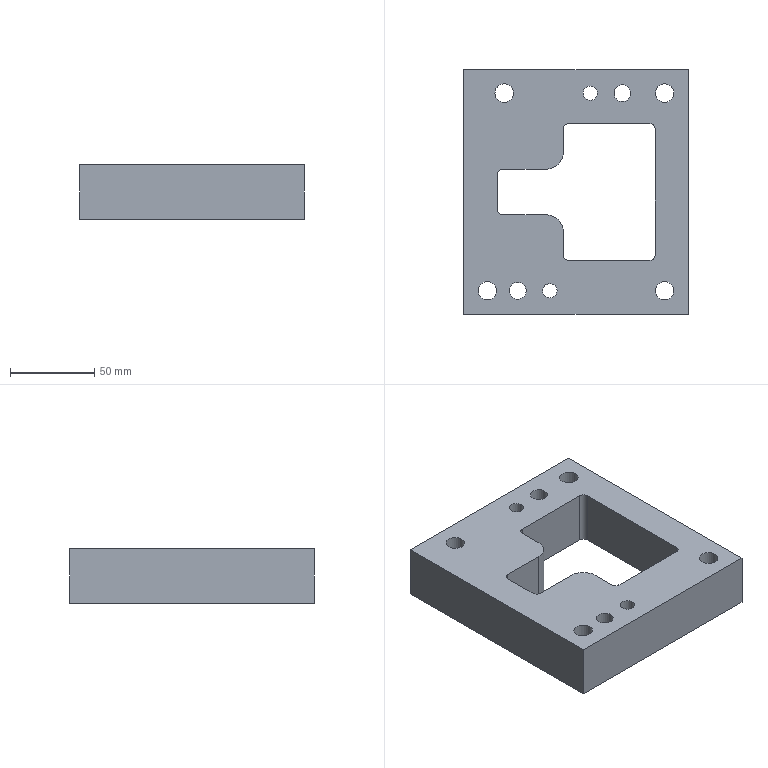Part | STEP file | lll_id3514_x_t | 1 solid | 38 faces | box 133 x 145 x 32 mm | volume 413987 mm3 | cylinder 20 | plane 18 | commonest cylinder face diameters 6 x6 11 x4 17 x4 8.506 x2 10 x2 20 x2
STEP:
#1=CARTESIAN_POINT('',(3776.,72.5,92.5));
#2=VERTEX_POINT('',#1);
#3=CARTESIAN_POINT('',(3909.,72.5,92.5));
#4=VERTEX_POINT('',#3);
#5=CARTESIAN_POINT('',(3841.5,72.5,92.5));
#6=DIRECTION('',(1.,0.,0.));
#7=VECTOR('',#6,1.);
#8=LINE('',#5,#7);
#9=EDGE_CURVE('',#2,#4,#8,.T.);
#10=ORIENTED_EDGE('',*,*,#9,.F.);
#11=CARTESIAN_POINT('',(3776.,-72.5,92.5));
#12=VERTEX_POINT('',#11);
#13=CARTESIAN_POINT('',(3776.,0.00007613,92.5));
#14=DIRECTION('',(0.,1.,0.));
#15=VECTOR('',#14,1.);
#16=LINE('',#13,#15);
#17=EDGE_CURVE('',#12,#2,#16,.T.);
#18=ORIENTED_EDGE('',*,*,#17,.F.);
#19=CARTESIAN_POINT('',(3909.,-72.5,92.5));
#20=VERTEX_POINT('',#19);
#21=CARTESIAN_POINT('',(3841.5,-72.5,92.5));
#22=DIRECTION('',(-1.,0.,0.));
#23=VECTOR('',#22,1.);
#24=LINE('',#21,#23);
#25=EDGE_CURVE('',#20,#12,#24,.T.);
#26=ORIENTED_EDGE('',*,*,#25,.F.);
#27=CARTESIAN_POINT('',(3909.,0.00007613,92.5));
#28=DIRECTION('',(0.,-1.,0.));
#29=VECTOR('',#28,1.);
#30=LINE('',#27,#29);
#31=EDGE_CURVE('',#4,#20,#30,.T.);
#32=ORIENTED_EDGE('',*,*,#31,.F.);
#33=EDGE_LOOP('',(#10,#18,#26,#32));
#34=FACE_BOUND('',#33,.T.);
#35=CARTESIAN_POINT('',(3889.5,58.5,92.5));
#36=VERTEX_POINT('',#35);
#37=CARTESIAN_POINT('',(3895.,58.5,92.5));
#38=DIRECTION('',(0.,0.,1.));
#39=DIRECTION('',(-1.,0.,0.));
#40=AXIS2_PLACEMENT_3D('',#37,#38,#39);
#41=CIRCLE('',#40,5.5);
#42=EDGE_CURVE('',#36,#36,#41,.T.);
#43=ORIENTED_EDGE('',*,*,#42,.F.);
#44=EDGE_LOOP('',(#43));
#45=FACE_BOUND('',#44,.T.);
#46=CARTESIAN_POINT('',(3784.5,-58.5,92.5));
#47=VERTEX_POINT('',#46);
#48=CARTESIAN_POINT('',(3790.,-58.5,92.5));
#49=DIRECTION('',(0.,0.,1.));
#50=DIRECTION('',(-1.,0.,0.));
#51=AXIS2_PLACEMENT_3D('',#48,#49,#50);
#52=CIRCLE('',#51,5.5);
#53=EDGE_CURVE('',#47,#47,#52,.T.);
#54=ORIENTED_EDGE('',*,*,#53,.F.);
#55=EDGE_LOOP('',(#54));
#56=FACE_BOUND('',#55,.T.);
#57=CARTESIAN_POINT('',(3794.5,58.5,92.5));
#58=VERTEX_POINT('',#57);
#59=CARTESIAN_POINT('',(3800.,58.5,92.5));
#60=DIRECTION('',(0.,0.,1.));
#61=DIRECTION('',(-1.,0.,0.));
#62=AXIS2_PLACEMENT_3D('',#59,#60,#61);
#63=CIRCLE('',#62,5.5);
#64=EDGE_CURVE('',#58,#58,#63,.T.);
#65=ORIENTED_EDGE('',*,*,#64,.F.);
#66=EDGE_LOOP('',(#65));
#67=FACE_BOUND('',#66,.T.);
#68=CARTESIAN_POINT('',(3889.5,-58.5,92.5));
#69=VERTEX_POINT('',#68);
#70=CARTESIAN_POINT('',(3895.,-58.5,92.5));
#71=DIRECTION('',(0.,0.,1.));
#72=DIRECTION('',(-1.,0.,0.));
#73=AXIS2_PLACEMENT_3D('',#70,#71,#72);
#74=CIRCLE('',#73,5.5);
#75=EDGE_CURVE('',#69,#69,#74,.T.);
#76=ORIENTED_EDGE('',*,*,#75,.F.);
#77=EDGE_LOOP('',(#76));
#78=FACE_BOUND('',#77,.T.);
#79=CARTESIAN_POINT('',(3865.,58.5,92.5));
#80=VERTEX_POINT('',#79);
#81=CARTESIAN_POINT('',(3870.,58.5,92.5));
#82=DIRECTION('',(0.,0.,1.));
#83=DIRECTION('',(-1.,0.,0.));
#84=AXIS2_PLACEMENT_3D('',#81,#82,#83);
#85=CIRCLE('',#84,5.);
#86=EDGE_CURVE('',#80,#80,#85,.T.);
#87=ORIENTED_EDGE('',*,*,#86,.F.);
#88=EDGE_LOOP('',(#87));
#89=FACE_BOUND('',#88,.T.);
#90=CARTESIAN_POINT('',(3803.,-58.5,92.5));
#91=VERTEX_POINT('',#90);
#92=CARTESIAN_POINT('',(3808.,-58.5,92.5));
#93=DIRECTION('',(0.,0.,1.));
#94=DIRECTION('',(-1.,0.,0.));
#95=AXIS2_PLACEMENT_3D('',#92,#93,#94);
#96=CIRCLE('',#95,5.);
#97=EDGE_CURVE('',#91,#91,#96,.T.);
#98=ORIENTED_EDGE('',*,*,#97,.F.);
#99=EDGE_LOOP('',(#98));
#100=FACE_BOUND('',#99,.T.);
#101=CARTESIAN_POINT('',(3846.747,58.5,92.5));
#102=VERTEX_POINT('',#101);
#103=CARTESIAN_POINT('',(3851.,58.5,92.5));
#104=DIRECTION('',(0.,0.,1.));
#105=DIRECTION('',(-1.,0.,0.));
#106=AXIS2_PLACEMENT_3D('',#103,#104,#105);
#107=CIRCLE('',#106,4.253);
#108=EDGE_CURVE('',#102,#102,#107,.T.);
#109=ORIENTED_EDGE('',*,*,#108,.F.);
#110=EDGE_LOOP('',(#109));
#111=FACE_BOUND('',#110,.T.);
#112=CARTESIAN_POINT('',(3822.747,-58.5,92.5));
#113=VERTEX_POINT('',#112);
#114=CARTESIAN_POINT('',(3827.,-58.5,92.5));
#115=DIRECTION('',(0.,0.,1.));
#116=DIRECTION('',(-1.,0.,0.));
#117=AXIS2_PLACEMENT_3D('',#114,#115,#116);
#118=CIRCLE('',#117,4.253);
#119=EDGE_CURVE('',#113,#113,#118,.T.);
#120=ORIENTED_EDGE('',*,*,#119,.F.);
#121=EDGE_LOOP('',(#120));
#122=FACE_BOUND('',#121,.T.);
#123=CARTESIAN_POINT('',(3796.,-10.5,92.5));
#124=VERTEX_POINT('',#123);
#125=CARTESIAN_POINT('',(3799.,-13.5,92.5));
#126=VERTEX_POINT('',#125);
#127=CARTESIAN_POINT('',(3799.,-10.5,92.5));
#128=DIRECTION('',(0.,0.,1.));
#129=DIRECTION('',(-1.,0.,0.));
#130=AXIS2_PLACEMENT_3D('',#127,#128,#129);
#131=CIRCLE('',#130,3.);
#132=EDGE_CURVE('',#124,#126,#131,.T.);
#133=ORIENTED_EDGE('',*,*,#132,.F.);
#134=CARTESIAN_POINT('',(3796.,10.5,92.5));
#135=VERTEX_POINT('',#134);
#136=CARTESIAN_POINT('',(3796.,236.7,92.5));
#137=DIRECTION('',(0.,1.,0.));
#138=VECTOR('',#137,1.);
#139=LINE('',#136,#138);
#140=EDGE_CURVE('',#124,#135,#139,.T.);
#141=ORIENTED_EDGE('',*,*,#140,.T.);
#142=CARTESIAN_POINT('',(3799.,13.5,92.5));
#143=VERTEX_POINT('',#142);
#144=CARTESIAN_POINT('',(3799.,10.5,92.5));
#145=DIRECTION('',(0.,0.,1.));
#146=DIRECTION('',(-1.,0.,0.));
#147=AXIS2_PLACEMENT_3D('',#144,#145,#146);
#148=CIRCLE('',#147,3.);
#149=EDGE_CURVE('',#143,#135,#148,.T.);
#150=ORIENTED_EDGE('',*,*,#149,.F.);
#151=CARTESIAN_POINT('',(3825.,13.5,92.5));
#152=VERTEX_POINT('',#151);
#153=CARTESIAN_POINT('',(3831.,13.5,92.5));
#154=DIRECTION('',(-1.,0.,0.));
#155=VECTOR('',#154,1.);
#156=LINE('',#153,#155);
#157=EDGE_CURVE('',#152,#143,#156,.T.);
#158=ORIENTED_EDGE('',*,*,#157,.F.);
#159=CARTESIAN_POINT('',(3835.,23.5,92.5));
#160=VERTEX_POINT('',#159);
#161=CARTESIAN_POINT('',(3825.,23.5,92.5));
#162=DIRECTION('',(0.,0.,-1.));
#163=DIRECTION('',(-1.,0.,0.));
#164=AXIS2_PLACEMENT_3D('',#161,#162,#163);
#165=CIRCLE('',#164,10.);
#166=EDGE_CURVE('',#160,#152,#165,.T.);
#167=ORIENTED_EDGE('',*,*,#166,.F.);
#168=CARTESIAN_POINT('',(3835.,37.5,92.5));
#169=VERTEX_POINT('',#168);
#170=CARTESIAN_POINT('',(3835.,38.,92.5));
#171=DIRECTION('',(0.,-1.,0.));
#172=VECTOR('',#171,1.);
#173=LINE('',#170,#172);
#174=EDGE_CURVE('',#169,#160,#173,.T.);
#175=ORIENTED_EDGE('',*,*,#174,.F.);
#176=CARTESIAN_POINT('',(3838.,40.5,92.5));
#177=VERTEX_POINT('',#176);
#178=CARTESIAN_POINT('',(3838.,37.5,92.5));
#179=DIRECTION('',(0.,0.,1.));
#180=DIRECTION('',(-1.,0.,0.));
#181=AXIS2_PLACEMENT_3D('',#178,#179,#180);
#182=CIRCLE('',#181,3.);
#183=EDGE_CURVE('',#177,#169,#182,.T.);
#184=ORIENTED_EDGE('',*,*,#183,.F.);
#185=CARTESIAN_POINT('',(3886.3,40.5,92.5));
#186=VERTEX_POINT('',#185);
#187=CARTESIAN_POINT('',(3587.234,40.5,92.5));
#188=DIRECTION('',(1.,0.,0.));
#189=VECTOR('',#188,1.);
#190=LINE('',#187,#189);
#191=EDGE_CURVE('',#177,#186,#190,.T.);
#192=ORIENTED_EDGE('',*,*,#191,.T.);
#193=CARTESIAN_POINT('',(3889.3,37.5,92.5));
#194=VERTEX_POINT('',#193);
#195=CARTESIAN_POINT('',(3886.3,37.5,92.5));
#196=DIRECTION('',(0.,0.,1.));
#197=DIRECTION('',(-1.,0.,0.));
#198=AXIS2_PLACEMENT_3D('',#195,#196,#197);
#199=CIRCLE('',#198,3.);
#200=EDGE_CURVE('',#194,#186,#199,.T.);
#201=ORIENTED_EDGE('',*,*,#200,.F.);
#202=CARTESIAN_POINT('',(3889.3,-37.5,92.5));
#203=VERTEX_POINT('',#202);
#204=CARTESIAN_POINT('',(3889.3,236.7,92.5));
#205=DIRECTION('',(0.,-1.,0.));
#206=VECTOR('',#205,1.);
#207=LINE('',#204,#206);
#208=EDGE_CURVE('',#194,#203,#207,.T.);
#209=ORIENTED_EDGE('',*,*,#208,.T.);
#210=CARTESIAN_POINT('',(3886.3,-40.5,92.5));
#211=VERTEX_POINT('',#210);
#212=CARTESIAN_POINT('',(3886.3,-37.5,92.5));
#213=DIRECTION('',(0.,0.,1.));
#214=DIRECTION('',(-1.,0.,0.));
#215=AXIS2_PLACEMENT_3D('',#212,#213,#214);
#216=CIRCLE('',#215,3.);
#217=EDGE_CURVE('',#211,#203,#216,.T.);
#218=ORIENTED_EDGE('',*,*,#217,.F.);
#219=CARTESIAN_POINT('',(3838.,-40.5,92.5));
#220=VERTEX_POINT('',#219);
#221=CARTESIAN_POINT('',(14362.883,-40.5,92.5));
#222=DIRECTION('',(1.,0.,0.));
#223=VECTOR('',#222,1.);
#224=LINE('',#221,#223);
#225=EDGE_CURVE('',#220,#211,#224,.T.);
#226=ORIENTED_EDGE('',*,*,#225,.F.);
#227=CARTESIAN_POINT('',(3835.,-37.5,92.5));
#228=VERTEX_POINT('',#227);
#229=CARTESIAN_POINT('',(3838.,-37.5,92.5));
#230=DIRECTION('',(0.,0.,1.));
#231=DIRECTION('',(-1.,0.,0.));
#232=AXIS2_PLACEMENT_3D('',#229,#230,#231);
#233=CIRCLE('',#232,3.);
#234=EDGE_CURVE('',#228,#220,#233,.T.);
#235=ORIENTED_EDGE('',*,*,#234,.F.);
#236=CARTESIAN_POINT('',(3835.,-23.5,92.5));
#237=VERTEX_POINT('',#236);
#238=CARTESIAN_POINT('',(3835.,236.7,92.5));
#239=DIRECTION('',(0.,1.,0.));
#240=VECTOR('',#239,1.);
#241=LINE('',#238,#240);
#242=EDGE_CURVE('',#228,#237,#241,.T.);
#243=ORIENTED_EDGE('',*,*,#242,.T.);
#244=CARTESIAN_POINT('',(3825.,-13.5,92.5));
#245=VERTEX_POINT('',#244);
#246=CARTESIAN_POINT('',(3825.,-23.5,92.5));
#247=DIRECTION('',(0.,0.,-1.));
#248=DIRECTION('',(-1.,0.,0.));
#249=AXIS2_PLACEMENT_3D('',#246,#247,#248);
#250=CIRCLE('',#249,10.);
#251=EDGE_CURVE('',#245,#237,#250,.T.);
#252=ORIENTED_EDGE('',*,*,#251,.F.);
#253=CARTESIAN_POINT('',(3587.234,-13.5,92.5));
#254=DIRECTION('',(-1.,0.,0.));
#255=VECTOR('',#254,1.);
#256=LINE('',#253,#255);
#257=EDGE_CURVE('',#245,#126,#256,.T.);
#258=ORIENTED_EDGE('',*,*,#257,.T.);
#259=EDGE_LOOP('',(#133,#141,#150,#158,#167,#175,#184,#192,#201,#209,#218,#226,#235,#243,#252,#258));
#260=FACE_BOUND('',#259,.T.);
#261=CARTESIAN_POINT('',(3841.5,0.00007613,92.5));
#262=DIRECTION('',(0.,0.,1.));
#263=DIRECTION('',(-1.,0.,0.));
#264=AXIS2_PLACEMENT_3D('',#261,#262,#263);
#265=PLANE('',#264);
#266=ADVANCED_FACE('',(#34,#45,#56,#67,#78,#89,#100,#111,#122,#260),#265,.T.);
#267=CARTESIAN_POINT('',(3889.3,-37.5,60.5));
#268=VERTEX_POINT('',#267);
#269=CARTESIAN_POINT('',(3886.3,-40.5,60.5));
#270=VERTEX_POINT('',#269);
#271=CARTESIAN_POINT('',(3886.3,-37.5,60.5));
#272=DIRECTION('',(0.,0.,-1.));
#273=DIRECTION('',(1.,0.,0.));
#274=AXIS2_PLACEMENT_3D('',#271,#272,#273);
#275=CIRCLE('',#274,3.);
#276=EDGE_CURVE('',#268,#270,#275,.T.);
#277=ORIENTED_EDGE('',*,*,#276,.F.);
#278=CARTESIAN_POINT('',(3889.3,37.5,60.5));
#279=VERTEX_POINT('',#278);
#280=CARTESIAN_POINT('',(3889.3,0.00007613,60.5));
#281=DIRECTION('',(0.,-1.,0.));
#282=VECTOR('',#281,1.);
#283=LINE('',#280,#282);
#284=EDGE_CURVE('',#279,#268,#283,.T.);
#285=ORIENTED_EDGE('',*,*,#284,.F.);
#286=CARTESIAN_POINT('',(3886.3,40.5,60.5));
#287=VERTEX_POINT('',#286);
#288=CARTESIAN_POINT('',(3886.3,37.5,60.5));
#289=DIRECTION('',(0.,0.,-1.));
#290=DIRECTION('',(1.,0.,0.));
#291=AXIS2_PLACEMENT_3D('',#288,#289,#290);
#292=CIRCLE('',#291,3.);
#293=EDGE_CURVE('',#287,#279,#292,.T.);
#294=ORIENTED_EDGE('',*,*,#293,.F.);
#295=CARTESIAN_POINT('',(3838.,40.5,60.5));
#296=VERTEX_POINT('',#295);
#297=CARTESIAN_POINT('',(3841.5,40.5,60.5));
#298=DIRECTION('',(1.,0.,0.));
#299=VECTOR('',#298,1.);
#300=LINE('',#297,#299);
#301=EDGE_CURVE('',#296,#287,#300,.T.);
#302=ORIENTED_EDGE('',*,*,#301,.F.);
#303=CARTESIAN_POINT('',(3835.,37.5,60.5));
#304=VERTEX_POINT('',#303);
#305=CARTESIAN_POINT('',(3838.,37.5,60.5));
#306=DIRECTION('',(0.,0.,-1.));
#307=DIRECTION('',(1.,0.,0.));
#308=AXIS2_PLACEMENT_3D('',#305,#306,#307);
#309=CIRCLE('',#308,3.);
#310=EDGE_CURVE('',#304,#296,#309,.T.);
#311=ORIENTED_EDGE('',*,*,#310,.F.);
#312=CARTESIAN_POINT('',(3835.,23.5,60.5));
#313=VERTEX_POINT('',#312);
#314=CARTESIAN_POINT('',(3835.,0.00007613,60.5));
#315=DIRECTION('',(0.,1.,0.));
#316=VECTOR('',#315,1.);
#317=LINE('',#314,#316);
#318=EDGE_CURVE('',#313,#304,#317,.T.);
#319=ORIENTED_EDGE('',*,*,#318,.F.);
#320=CARTESIAN_POINT('',(3825.,13.5,60.5));
#321=VERTEX_POINT('',#320);
#322=CARTESIAN_POINT('',(3825.,23.5,60.5));
#323=DIRECTION('',(0.,0.,-1.));
#324=DIRECTION('',(1.,0.,0.));
#325=AXIS2_PLACEMENT_3D('',#322,#323,#324);
#326=CIRCLE('',#325,10.);
#327=EDGE_CURVE('',#313,#321,#326,.T.);
#328=ORIENTED_EDGE('',*,*,#327,.T.);
#329=CARTESIAN_POINT('',(3799.,13.5,60.5));
#330=VERTEX_POINT('',#329);
#331=CARTESIAN_POINT('',(3841.5,13.5,60.5));
#332=DIRECTION('',(1.,0.,0.));
#333=VECTOR('',#332,1.);
#334=LINE('',#331,#333);
#335=EDGE_CURVE('',#330,#321,#334,.T.);
#336=ORIENTED_EDGE('',*,*,#335,.F.);
#337=CARTESIAN_POINT('',(3796.,10.5,60.5));
#338=VERTEX_POINT('',#337);
#339=CARTESIAN_POINT('',(3799.,10.5,60.5));
#340=DIRECTION('',(0.,0.,-1.));
#341=DIRECTION('',(1.,0.,0.));
#342=AXIS2_PLACEMENT_3D('',#339,#340,#341);
#343=CIRCLE('',#342,3.);
#344=EDGE_CURVE('',#338,#330,#343,.T.);
#345=ORIENTED_EDGE('',*,*,#344,.F.);
#346=CARTESIAN_POINT('',(3796.,-10.5,60.5));
#347=VERTEX_POINT('',#346);
#348=CARTESIAN_POINT('',(3796.,0.00007613,60.5));
#349=DIRECTION('',(0.,1.,0.));
#350=VECTOR('',#349,1.);
#351=LINE('',#348,#350);
#352=EDGE_CURVE('',#347,#338,#351,.T.);
#353=ORIENTED_EDGE('',*,*,#352,.F.);
#354=CARTESIAN_POINT('',(3799.,-13.5,60.5));
#355=VERTEX_POINT('',#354);
#356=CARTESIAN_POINT('',(3799.,-10.5,60.5));
#357=DIRECTION('',(0.,0.,-1.));
#358=DIRECTION('',(1.,0.,0.));
#359=AXIS2_PLACEMENT_3D('',#356,#357,#358);
#360=CIRCLE('',#359,3.);
#361=EDGE_CURVE('',#355,#347,#360,.T.);
#362=ORIENTED_EDGE('',*,*,#361,.F.);
#363=CARTESIAN_POINT('',(3825.,-13.5,60.5));
#364=VERTEX_POINT('',#363);
#365=CARTESIAN_POINT('',(3841.5,-13.5,60.5));
#366=DIRECTION('',(-1.,0.,0.));
#367=VECTOR('',#366,1.);
#368=LINE('',#365,#367);
#369=EDGE_CURVE('',#364,#355,#368,.T.);
#370=ORIENTED_EDGE('',*,*,#369,.F.);
#371=CARTESIAN_POINT('',(3835.,-23.5,60.5));
#372=VERTEX_POINT('',#371);
#373=CARTESIAN_POINT('',(3825.,-23.5,60.5));
#374=DIRECTION('',(0.,0.,-1.));
#375=DIRECTION('',(1.,0.,0.));
#376=AXIS2_PLACEMENT_3D('',#373,#374,#375);
#377=CIRCLE('',#376,10.);
#378=EDGE_CURVE('',#364,#372,#377,.T.);
#379=ORIENTED_EDGE('',*,*,#378,.T.);
#380=CARTESIAN_POINT('',(3835.,-37.5,60.5));
#381=VERTEX_POINT('',#380);
#382=CARTESIAN_POINT('',(3835.,0.00007613,60.5));
#383=DIRECTION('',(0.,1.,0.));
#384=VECTOR('',#383,1.);
#385=LINE('',#382,#384);
#386=EDGE_CURVE('',#381,#372,#385,.T.);
#387=ORIENTED_EDGE('',*,*,#386,.F.);
#388=CARTESIAN_POINT('',(3838.,-40.5,60.5));
#389=VERTEX_POINT('',#388);
#390=CARTESIAN_POINT('',(3838.,-37.5,60.5));
#391=DIRECTION('',(0.,0.,-1.));
#392=DIRECTION('',(1.,0.,0.));
#393=AXIS2_PLACEMENT_3D('',#390,#391,#392);
#394=CIRCLE('',#393,3.);
#395=EDGE_CURVE('',#389,#381,#394,.T.);
#396=ORIENTED_EDGE('',*,*,#395,.F.);
#397=CARTESIAN_POINT('',(3841.5,-40.5,60.5));
#398=DIRECTION('',(-1.,0.,0.));
#399=VECTOR('',#398,1.);
#400=LINE('',#397,#399);
#401=EDGE_CURVE('',#270,#389,#400,.T.);
#402=ORIENTED_EDGE('',*,*,#401,.F.);
#403=EDGE_LOOP('',(#277,#285,#294,#302,#311,#319,#328,#336,#345,#353,#362,#370,#379,#387,#396,#402));
#404=FACE_BOUND('',#403,.T.);
#405=CARTESIAN_POINT('',(3846.747,58.5,60.5));
#406=VERTEX_POINT('',#405);
#407=CARTESIAN_POINT('',(3851.,58.5,60.5));
#408=DIRECTION('',(0.,0.,1.));
#409=DIRECTION('',(-1.,0.,0.));
#410=AXIS2_PLACEMENT_3D('',#407,#408,#409);
#411=CIRCLE('',#410,4.253);
#412=EDGE_CURVE('',#406,#406,#411,.T.);
#413=ORIENTED_EDGE('',*,*,#412,.T.);
#414=EDGE_LOOP('',(#413));
#415=FACE_BOUND('',#414,.T.);
#416=CARTESIAN_POINT('',(3813.,-58.5,60.5));
#417=VERTEX_POINT('',#416);
#418=CARTESIAN_POINT('',(3808.,-58.5,60.5));
#419=DIRECTION('',(0.,0.,-1.));
#420=DIRECTION('',(1.,0.,0.));
#421=AXIS2_PLACEMENT_3D('',#418,#419,#420);
#422=CIRCLE('',#421,5.);
#423=EDGE_CURVE('',#417,#417,#422,.T.);
#424=ORIENTED_EDGE('',*,*,#423,.F.);
#425=EDGE_LOOP('',(#424));
#426=FACE_BOUND('',#425,.T.);
#427=CARTESIAN_POINT('',(3875.,58.5,60.5));
#428=VERTEX_POINT('',#427);
#429=CARTESIAN_POINT('',(3870.,58.5,60.5));
#430=DIRECTION('',(0.,0.,-1.));
#431=DIRECTION('',(1.,0.,0.));
#432=AXIS2_PLACEMENT_3D('',#429,#430,#431);
#433=CIRCLE('',#432,5.);
#434=EDGE_CURVE('',#428,#428,#433,.T.);
#435=ORIENTED_EDGE('',*,*,#434,.F.);
#436=EDGE_LOOP('',(#435));
#437=FACE_BOUND('',#436,.T.);
#438=CARTESIAN_POINT('',(3808.5,58.5,60.5));
#439=VERTEX_POINT('',#438);
#440=CARTESIAN_POINT('',(3800.,58.5,60.5));
#441=DIRECTION('',(0.,0.,1.));
#442=DIRECTION('',(1.,0.,0.));
#443=AXIS2_PLACEMENT_3D('',#440,#441,#442);
#444=CIRCLE('',#443,8.5);
#445=EDGE_CURVE('',#439,#439,#444,.T.);
#446=ORIENTED_EDGE('',*,*,#445,.T.);
#447=EDGE_LOOP('',(#446));
#448=FACE_BOUND('',#447,.T.);
#449=CARTESIAN_POINT('',(3903.5,58.5,60.5));
#450=VERTEX_POINT('',#449);
#451=CARTESIAN_POINT('',(3895.,58.5,60.5));
#452=DIRECTION('',(0.,0.,1.));
#453=DIRECTION('',(1.,0.,0.));
#454=AXIS2_PLACEMENT_3D('',#451,#452,#453);
#455=CIRCLE('',#454,8.5);
#456=EDGE_CURVE('',#450,#450,#455,.T.);
#457=ORIENTED_EDGE('',*,*,#456,.T.);
#458=EDGE_LOOP('',(#457));
#459=FACE_BOUND('',#458,.T.);
#460=CARTESIAN_POINT('',(3776.,72.5,60.5));
#461=VERTEX_POINT('',#460);
#462=CARTESIAN_POINT('',(3776.,-72.5,60.5));
#463=VERTEX_POINT('',#462);
#464=CARTESIAN_POINT('',(3776.,0.00007613,60.5));
#465=DIRECTION('',(0.,-1.,0.));
#466=VECTOR('',#465,1.);
#467=LINE('',#464,#466);
#468=EDGE_CURVE('',#461,#463,#467,.T.);
#469=ORIENTED_EDGE('',*,*,#468,.F.);
#470=CARTESIAN_POINT('',(3909.,72.5,60.5));
#471=VERTEX_POINT('',#470);
#472=CARTESIAN_POINT('',(3841.5,72.5,60.5));
#473=DIRECTION('',(-1.,0.,0.));
#474=VECTOR('',#473,1.);
#475=LINE('',#472,#474);
#476=EDGE_CURVE('',#471,#461,#475,.T.);
#477=ORIENTED_EDGE('',*,*,#476,.F.);
#478=CARTESIAN_POINT('',(3909.,-72.5,60.5));
#479=VERTEX_POINT('',#478);
#480=CARTESIAN_POINT('',(3909.,0.00007613,60.5));
#481=DIRECTION('',(0.,1.,0.));
#482=VECTOR('',#481,1.);
#483=LINE('',#480,#482);
#484=EDGE_CURVE('',#479,#471,#483,.T.);
#485=ORIENTED_EDGE('',*,*,#484,.F.);
#486=CARTESIAN_POINT('',(3841.5,-72.5,60.5));
#487=DIRECTION('',(1.,0.,0.));
#488=VECTOR('',#487,1.);
#489=LINE('',#486,#488);
#490=EDGE_CURVE('',#463,#479,#489,.T.);
#491=ORIENTED_EDGE('',*,*,#490,.F.);
#492=EDGE_LOOP('',(#469,#477,#485,#491));
#493=FACE_BOUND('',#492,.T.);
#494=CARTESIAN_POINT('',(3798.5,-58.5,60.5));
#495=VERTEX_POINT('',#494);
#496=CARTESIAN_POINT('',(3790.,-58.5,60.5));
#497=DIRECTION('',(0.,0.,1.));
#498=DIRECTION('',(1.,0.,0.));
#499=AXIS2_PLACEMENT_3D('',#496,#497,#498);
#500=CIRCLE('',#499,8.5);
#501=EDGE_CURVE('',#495,#495,#500,.T.);
#502=ORIENTED_EDGE('',*,*,#501,.T.);
#503=EDGE_LOOP('',(#502));
#504=FACE_BOUND('',#503,.T.);
#505=CARTESIAN_POINT('',(3903.5,-58.5,60.5));
#506=VERTEX_POINT('',#505);
#507=CARTESIAN_POINT('',(3895.,-58.5,60.5));
#508=DIRECTION('',(0.,0.,1.));
#509=DIRECTION('',(1.,0.,0.));
#510=AXIS2_PLACEMENT_3D('',#507,#508,#509);
#511=CIRCLE('',#510,8.5);
#512=EDGE_CURVE('',#506,#506,#511,.T.);
#513=ORIENTED_EDGE('',*,*,#512,.T.);
#514=EDGE_LOOP('',(#513));
#515=FACE_BOUND('',#514,.T.);
#516=CARTESIAN_POINT('',(3822.747,-58.5,60.5));
#517=VERTEX_POINT('',#516);
#518=CARTESIAN_POINT('',(3827.,-58.5,60.5));
#519=DIRECTION('',(0.,0.,1.));
#520=DIRECTION('',(-1.,0.,0.));
#521=AXIS2_PLACEMENT_3D('',#518,#519,#520);
#522=CIRCLE('',#521,4.253);
#523=EDGE_CURVE('',#517,#517,#522,.T.);
#524=ORIENTED_EDGE('',*,*,#523,.T.);
#525=EDGE_LOOP('',(#524));
#526=FACE_BOUND('',#525,.T.);
#527=CARTESIAN_POINT('',(3841.5,0.00007613,60.5));
#528=DIRECTION('',(0.,0.,-1.));
#529=DIRECTION('',(1.,0.,0.));
#530=AXIS2_PLACEMENT_3D('',#527,#528,#529);
#531=PLANE('',#530);
#532=ADVANCED_FACE('',(#404,#415,#426,#437,#448,#459,#493,#504,#515,#526),#531,.T.);
#533=CARTESIAN_POINT('',(3776.,72.5,60.5));
#534=DIRECTION('',(0.,0.,1.));
#535=VECTOR('',#534,1.);
#536=LINE('',#533,#535);
#537=EDGE_CURVE('',#461,#2,#536,.T.);
#538=ORIENTED_EDGE('',*,*,#537,.T.);
#539=ORIENTED_EDGE('',*,*,#9,.T.);
#540=CARTESIAN_POINT('',(3909.,72.5,60.5));
#541=DIRECTION('',(0.,0.,1.));
#542=VECTOR('',#541,1.);
#543=LINE('',#540,#542);
#544=EDGE_CURVE('',#471,#4,#543,.T.);
#545=ORIENTED_EDGE('',*,*,#544,.F.);
#546=ORIENTED_EDGE('',*,*,#476,.T.);
#547=EDGE_LOOP('',(#538,#539,#545,#546));
#548=FACE_OUTER_BOUND('',#547,.T.);
#549=CARTESIAN_POINT('',(3841.5,72.5,60.5));
#550=DIRECTION('',(0.,1.,0.));
#551=DIRECTION('',(0.,0.,-1.));
#552=AXIS2_PLACEMENT_3D('',#549,#550,#551);
#553=PLANE('',#552);
#554=ADVANCED_FACE('',(#548),#553,.T.);
#555=ORIENTED_EDGE('',*,*,#544,.T.);
#556=ORIENTED_EDGE('',*,*,#31,.T.);
#557=CARTESIAN_POINT('',(3909.,-72.5,60.5));
#558=DIRECTION('',(0.,0.,1.));
#559=VECTOR('',#558,1.);
#560=LINE('',#557,#559);
#561=EDGE_CURVE('',#479,#20,#560,.T.);
#562=ORIENTED_EDGE('',*,*,#561,.F.);
#563=ORIENTED_EDGE('',*,*,#484,.T.);
#564=EDGE_LOOP('',(#555,#556,#562,#563));
#565=FACE_OUTER_BOUND('',#564,.T.);
#566=CARTESIAN_POINT('',(3909.,0.00007613,60.5));
#567=DIRECTION('',(1.,0.,0.));
#568=DIRECTION('',(0.,0.,1.));
#569=AXIS2_PLACEMENT_3D('',#566,#567,#568);
#570=PLANE('',#569);
#571=ADVANCED_FACE('',(#565),#570,.T.);
#572=ORIENTED_EDGE('',*,*,#561,.T.);
#573=ORIENTED_EDGE('',*,*,#25,.T.);
#574=CARTESIAN_POINT('',(3776.,-72.5,60.5));
#575=DIRECTION('',(0.,0.,1.));
#576=VECTOR('',#575,1.);
#577=LINE('',#574,#576);
#578=EDGE_CURVE('',#463,#12,#577,.T.);
#579=ORIENTED_EDGE('',*,*,#578,.F.);
#580=ORIENTED_EDGE('',*,*,#490,.T.);
#581=EDGE_LOOP('',(#572,#573,#579,#580));
#582=FACE_OUTER_BOUND('',#581,.T.);
#583=CARTESIAN_POINT('',(3841.5,-72.5,60.5));
#584=DIRECTION('',(0.,-1.,0.));
#585=DIRECTION('',(0.,0.,1.));
#586=AXIS2_PLACEMENT_3D('',#583,#584,#585);
#587=PLANE('',#586);
#588=ADVANCED_FACE('',(#582),#587,.T.);
#589=ORIENTED_EDGE('',*,*,#468,.T.);
#590=ORIENTED_EDGE('',*,*,#578,.T.);
#591=ORIENTED_EDGE('',*,*,#17,.T.);
#592=ORIENTED_EDGE('',*,*,#537,.F.);
#593=EDGE_LOOP('',(#589,#590,#591,#592));
#594=FACE_OUTER_BOUND('',#593,.T.);
#595=CARTESIAN_POINT('',(3776.,0.00007613,60.5));
#596=DIRECTION('',(-1.,0.,0.));
#597=DIRECTION('',(0.,0.,-1.));
#598=AXIS2_PLACEMENT_3D('',#595,#596,#597);
#599=PLANE('',#598);
#600=ADVANCED_FACE('',(#594),#599,.T.);
#601=ORIENTED_EDGE('',*,*,#42,.T.);
#602=EDGE_LOOP('',(#601));
#603=FACE_BOUND('',#602,.T.);
#604=CARTESIAN_POINT('',(3889.5,58.5,73.5));
#605=VERTEX_POINT('',#604);
#606=CARTESIAN_POINT('',(3895.,58.5,73.5));
#607=DIRECTION('',(0.,0.,1.));
#608=DIRECTION('',(-1.,0.,0.));
#609=AXIS2_PLACEMENT_3D('',#606,#607,#608);
#610=CIRCLE('',#609,5.5);
#611=EDGE_CURVE('',#605,#605,#610,.T.);
#612=ORIENTED_EDGE('',*,*,#611,.F.);
#613=EDGE_LOOP('',(#612));
#614=FACE_BOUND('',#613,.T.);
#615=CARTESIAN_POINT('',(3895.,58.5,57.5));
#616=DIRECTION('',(0.,0.,1.));
#617=DIRECTION('',(-1.,0.,0.));
#618=AXIS2_PLACEMENT_3D('',#615,#616,#617);
#619=CYLINDRICAL_SURFACE('',#618,5.5);
#620=ADVANCED_FACE('',(#603,#614),#619,.F.);
#621=ORIENTED_EDGE('',*,*,#611,.T.);
#622=EDGE_LOOP('',(#621));
#623=FACE_BOUND('',#622,.T.);
#624=CARTESIAN_POINT('',(3886.5,58.5,73.5));
#625=VERTEX_POINT('',#624);
#626=CARTESIAN_POINT('',(3895.,58.5,73.5));
#627=DIRECTION('',(0.,0.,1.));
#628=DIRECTION('',(-1.,0.,0.));
#629=AXIS2_PLACEMENT_3D('',#626,#627,#628);
#630=CIRCLE('',#629,8.5);
#631=EDGE_CURVE('',#625,#625,#630,.T.);
#632=ORIENTED_EDGE('',*,*,#631,.F.);
#633=EDGE_LOOP('',(#632));
#634=FACE_BOUND('',#633,.T.);
#635=CARTESIAN_POINT('',(3895.,58.5,73.5));
#636=DIRECTION('',(0.,0.,1.));
#637=DIRECTION('',(-1.,0.,0.));
#638=AXIS2_PLACEMENT_3D('',#635,#636,#637);
#639=PLANE('',#638);
#640=ADVANCED_FACE('',(#623,#634),#639,.F.);
#641=ORIENTED_EDGE('',*,*,#631,.T.);
#642=EDGE_LOOP('',(#641));
#643=FACE_BOUND('',#642,.T.);
#644=ORIENTED_EDGE('',*,*,#456,.F.);
#645=EDGE_LOOP('',(#644));
#646=FACE_BOUND('',#645,.T.);
#647=CARTESIAN_POINT('',(3895.,58.5,60.5));
#648=DIRECTION('',(0.,0.,1.));
#649=DIRECTION('',(-1.,0.,0.));
#650=AXIS2_PLACEMENT_3D('',#647,#648,#649);
#651=CYLINDRICAL_SURFACE('',#650,8.5);
#652=ADVANCED_FACE('',(#643,#646),#651,.F.);
#653=ORIENTED_EDGE('',*,*,#53,.T.);
#654=EDGE_LOOP('',(#653));
#655=FACE_BOUND('',#654,.T.);
#656=CARTESIAN_POINT('',(3784.5,-58.5,73.5));
#657=VERTEX_POINT('',#656);
#658=CARTESIAN_POINT('',(3790.,-58.5,73.5));
#659=DIRECTION('',(0.,0.,1.));
#660=DIRECTION('',(-1.,0.,0.));
#661=AXIS2_PLACEMENT_3D('',#658,#659,#660);
#662=CIRCLE('',#661,5.5);
#663=EDGE_CURVE('',#657,#657,#662,.T.);
#664=ORIENTED_EDGE('',*,*,#663,.F.);
#665=EDGE_LOOP('',(#664));
#666=FACE_BOUND('',#665,.T.);
#667=CARTESIAN_POINT('',(3790.,-58.5,57.5));
#668=DIRECTION('',(0.,0.,1.));
#669=DIRECTION('',(-1.,0.,0.));
#670=AXIS2_PLACEMENT_3D('',#667,#668,#669);
#671=CYLINDRICAL_SURFACE('',#670,5.5);
#672=ADVANCED_FACE('',(#655,#666),#671,.F.);
#673=ORIENTED_EDGE('',*,*,#663,.T.);
#674=EDGE_LOOP('',(#673));
#675=FACE_BOUND('',#674,.T.);
#676=CARTESIAN_POINT('',(3781.5,-58.5,73.5));
#677=VERTEX_POINT('',#676);
#678=CARTESIAN_POINT('',(3790.,-58.5,73.5));
#679=DIRECTION('',(0.,0.,1.));
#680=DIRECTION('',(-1.,0.,0.));
#681=AXIS2_PLACEMENT_3D('',#678,#679,#680);
#682=CIRCLE('',#681,8.5);
#683=EDGE_CURVE('',#677,#677,#682,.T.);
#684=ORIENTED_EDGE('',*,*,#683,.F.);
#685=EDGE_LOOP('',(#684));
#686=FACE_BOUND('',#685,.T.);
#687=CARTESIAN_POINT('',(3790.,-58.5,73.5));
#688=DIRECTION('',(0.,0.,1.));
#689=DIRECTION('',(-1.,0.,0.));
#690=AXIS2_PLACEMENT_3D('',#687,#688,#689);
#691=PLANE('',#690);
#692=ADVANCED_FACE('',(#675,#686),#691,.F.);
#693=ORIENTED_EDGE('',*,*,#683,.T.);
#694=EDGE_LOOP('',(#693));
#695=FACE_BOUND('',#694,.T.);
#696=ORIENTED_EDGE('',*,*,#501,.F.);
#697=EDGE_LOOP('',(#696));
#698=FACE_BOUND('',#697,.T.);
#699=CARTESIAN_POINT('',(3790.,-58.5,60.5));
#700=DIRECTION('',(0.,0.,1.));
#701=DIRECTION('',(-1.,0.,0.));
#702=AXIS2_PLACEMENT_3D('',#699,#700,#701);
#703=CYLINDRICAL_SURFACE('',#702,8.5);
#704=ADVANCED_FACE('',(#695,#698),#703,.F.);
#705=ORIENTED_EDGE('',*,*,#64,.T.);
#706=EDGE_LOOP('',(#705));
#707=FACE_BOUND('',#706,.T.);
#708=CARTESIAN_POINT('',(3794.5,58.5,73.5));
#709=VERTEX_POINT('',#708);
#710=CARTESIAN_POINT('',(3800.,58.5,73.5));
#711=DIRECTION('',(0.,0.,1.));
#712=DIRECTION('',(-1.,0.,0.));
#713=AXIS2_PLACEMENT_3D('',#710,#711,#712);
#714=CIRCLE('',#713,5.5);
#715=EDGE_CURVE('',#709,#709,#714,.T.);
#716=ORIENTED_EDGE('',*,*,#715,.F.);
#717=EDGE_LOOP('',(#716));
#718=FACE_BOUND('',#717,.T.);
#719=CARTESIAN_POINT('',(3800.,58.5,57.5));
#720=DIRECTION('',(0.,0.,1.));
#721=DIRECTION('',(-1.,0.,0.));
#722=AXIS2_PLACEMENT_3D('',#719,#720,#721);
#723=CYLINDRICAL_SURFACE('',#722,5.5);
#724=ADVANCED_FACE('',(#707,#718),#723,.F.);
#725=ORIENTED_EDGE('',*,*,#715,.T.);
#726=EDGE_LOOP('',(#725));
#727=FACE_BOUND('',#726,.T.);
#728=CARTESIAN_POINT('',(3791.5,58.5,73.5));
#729=VERTEX_POINT('',#728);
#730=CARTESIAN_POINT('',(3800.,58.5,73.5));
#731=DIRECTION('',(0.,0.,1.));
#732=DIRECTION('',(-1.,0.,0.));
#733=AXIS2_PLACEMENT_3D('',#730,#731,#732);
#734=CIRCLE('',#733,8.5);
#735=EDGE_CURVE('',#729,#729,#734,.T.);
#736=ORIENTED_EDGE('',*,*,#735,.F.);
#737=EDGE_LOOP('',(#736));
#738=FACE_BOUND('',#737,.T.);
#739=CARTESIAN_POINT('',(3800.,58.5,73.5));
#740=DIRECTION('',(0.,0.,1.));
#741=DIRECTION('',(-1.,0.,0.));
#742=AXIS2_PLACEMENT_3D('',#739,#740,#741);
#743=PLANE('',#742);
#744=ADVANCED_FACE('',(#727,#738),#743,.F.);
#745=ORIENTED_EDGE('',*,*,#735,.T.);
#746=EDGE_LOOP('',(#745));
#747=FACE_BOUND('',#746,.T.);
#748=ORIENTED_EDGE('',*,*,#445,.F.);
#749=EDGE_LOOP('',(#748));
#750=FACE_BOUND('',#749,.T.);
#751=CARTESIAN_POINT('',(3800.,58.5,60.5));
#752=DIRECTION('',(0.,0.,1.));
#753=DIRECTION('',(-1.,0.,0.));
#754=AXIS2_PLACEMENT_3D('',#751,#752,#753);
#755=CYLINDRICAL_SURFACE('',#754,8.5);
#756=ADVANCED_FACE('',(#747,#750),#755,.F.);
#757=ORIENTED_EDGE('',*,*,#75,.T.);
#758=EDGE_LOOP('',(#757));
#759=FACE_BOUND('',#758,.T.);
#760=CARTESIAN_POINT('',(3889.5,-58.5,73.5));
#761=VERTEX_POINT('',#760);
#762=CARTESIAN_POINT('',(3895.,-58.5,73.5));
#763=DIRECTION('',(0.,0.,1.));
#764=DIRECTION('',(-1.,0.,0.));
#765=AXIS2_PLACEMENT_3D('',#762,#763,#764);
#766=CIRCLE('',#765,5.5);
#767=EDGE_CURVE('',#761,#761,#766,.T.);
#768=ORIENTED_EDGE('',*,*,#767,.F.);
#769=EDGE_LOOP('',(#768));
#770=FACE_BOUND('',#769,.T.);
#771=CARTESIAN_POINT('',(3895.,-58.5,57.5));
#772=DIRECTION('',(0.,0.,1.));
#773=DIRECTION('',(-1.,0.,0.));
#774=AXIS2_PLACEMENT_3D('',#771,#772,#773);
#775=CYLINDRICAL_SURFACE('',#774,5.5);
#776=ADVANCED_FACE('',(#759,#770),#775,.F.);
#777=ORIENTED_EDGE('',*,*,#767,.T.);
#778=EDGE_LOOP('',(#777));
#779=FACE_BOUND('',#778,.T.);
#780=CARTESIAN_POINT('',(3886.5,-58.5,73.5));
#781=VERTEX_POINT('',#780);
#782=CARTESIAN_POINT('',(3895.,-58.5,73.5));
#783=DIRECTION('',(0.,0.,1.));
#784=DIRECTION('',(-1.,0.,0.));
#785=AXIS2_PLACEMENT_3D('',#782,#783,#784);
#786=CIRCLE('',#785,8.5);
#787=EDGE_CURVE('',#781,#781,#786,.T.);
#788=ORIENTED_EDGE('',*,*,#787,.F.);
#789=EDGE_LOOP('',(#788));
#790=FACE_BOUND('',#789,.T.);
#791=CARTESIAN_POINT('',(3895.,-58.5,73.5));
#792=DIRECTION('',(0.,0.,1.));
#793=DIRECTION('',(-1.,0.,0.));
#794=AXIS2_PLACEMENT_3D('',#791,#792,#793);
#795=PLANE('',#794);
#796=ADVANCED_FACE('',(#779,#790),#795,.F.);
#797=ORIENTED_EDGE('',*,*,#787,.T.);
#798=EDGE_LOOP('',(#797));
#799=FACE_BOUND('',#798,.T.);
#800=ORIENTED_EDGE('',*,*,#512,.F.);
#801=EDGE_LOOP('',(#800));
#802=FACE_BOUND('',#801,.T.);
#803=CARTESIAN_POINT('',(3895.,-58.5,60.5));
#804=DIRECTION('',(0.,0.,1.));
#805=DIRECTION('',(-1.,0.,0.));
#806=AXIS2_PLACEMENT_3D('',#803,#804,#805);
#807=CYLINDRICAL_SURFACE('',#806,8.5);
#808=ADVANCED_FACE('',(#799,#802),#807,.F.);
#809=ORIENTED_EDGE('',*,*,#434,.T.);
#810=EDGE_LOOP('',(#809));
#811=FACE_BOUND('',#810,.T.);
#812=ORIENTED_EDGE('',*,*,#86,.T.);
#813=EDGE_LOOP('',(#812));
#814=FACE_BOUND('',#813,.T.);
#815=CARTESIAN_POINT('',(3870.,58.5,57.5));
#816=DIRECTION('',(0.,0.,1.));
#817=DIRECTION('',(-1.,0.,0.));
#818=AXIS2_PLACEMENT_3D('',#815,#816,#817);
#819=CYLINDRICAL_SURFACE('',#818,5.);
#820=ADVANCED_FACE('',(#811,#814),#819,.F.);
#821=ORIENTED_EDGE('',*,*,#423,.T.);
#822=EDGE_LOOP('',(#821));
#823=FACE_BOUND('',#822,.T.);
#824=ORIENTED_EDGE('',*,*,#97,.T.);
#825=EDGE_LOOP('',(#824));
#826=FACE_BOUND('',#825,.T.);
#827=CARTESIAN_POINT('',(3808.,-58.5,57.5));
#828=DIRECTION('',(0.,0.,1.));
#829=DIRECTION('',(-1.,0.,0.));
#830=AXIS2_PLACEMENT_3D('',#827,#828,#829);
#831=CYLINDRICAL_SURFACE('',#830,5.);
#832=ADVANCED_FACE('',(#823,#826),#831,.F.);
#833=ORIENTED_EDGE('',*,*,#108,.T.);
#834=EDGE_LOOP('',(#833));
#835=FACE_BOUND('',#834,.T.);
#836=ORIENTED_EDGE('',*,*,#412,.F.);
#837=EDGE_LOOP('',(#836));
#838=FACE_BOUND('',#837,.T.);
#839=CARTESIAN_POINT('',(3851.,58.5,60.5));
#840=DIRECTION('',(0.,0.,1.));
#841=DIRECTION('',(-1.,0.,0.));
#842=AXIS2_PLACEMENT_3D('',#839,#840,#841);
#843=CYLINDRICAL_SURFACE('',#842,4.253);
#844=ADVANCED_FACE('',(#835,#838),#843,.F.);
#845=ORIENTED_EDGE('',*,*,#119,.T.);
#846=EDGE_LOOP('',(#845));
#847=FACE_BOUND('',#846,.T.);
#848=ORIENTED_EDGE('',*,*,#523,.F.);
#849=EDGE_LOOP('',(#848));
#850=FACE_BOUND('',#849,.T.);
#851=CARTESIAN_POINT('',(3827.,-58.5,60.5));
#852=DIRECTION('',(0.,0.,1.));
#853=DIRECTION('',(-1.,0.,0.));
#854=AXIS2_PLACEMENT_3D('',#851,#852,#853);
#855=CYLINDRICAL_SURFACE('',#854,4.253);
#856=ADVANCED_FACE('',(#847,#850),#855,.F.);
#857=CARTESIAN_POINT('',(3825.,-13.5,2.5));
#858=DIRECTION('',(0.,0.,-1.));
#859=VECTOR('',#858,1.);
#860=LINE('',#857,#859);
#861=EDGE_CURVE('',#245,#364,#860,.T.);
#862=ORIENTED_EDGE('',*,*,#861,.F.);
#863=ORIENTED_EDGE('',*,*,#251,.T.);
#864=CARTESIAN_POINT('',(3835.,-23.5,2.5));
#865=DIRECTION('',(0.,0.,1.));
#866=VECTOR('',#865,1.);
#867=LINE('',#864,#866);
#868=EDGE_CURVE('',#372,#237,#867,.T.);
#869=ORIENTED_EDGE('',*,*,#868,.F.);
#870=ORIENTED_EDGE('',*,*,#378,.F.);
#871=EDGE_LOOP('',(#862,#863,#869,#870));
#872=FACE_OUTER_BOUND('',#871,.T.);
#873=CARTESIAN_POINT('',(3825.,-23.5,2.5));
#874=DIRECTION('',(0.,0.,1.));
#875=DIRECTION('',(-1.,0.,0.));
#876=AXIS2_PLACEMENT_3D('',#873,#874,#875);
#877=CYLINDRICAL_SURFACE('',#876,10.);
#878=ADVANCED_FACE('',(#872),#877,.T.);
#879=ORIENTED_EDGE('',*,*,#395,.T.);
#880=CARTESIAN_POINT('',(3835.,-37.5,2.5));
#881=DIRECTION('',(0.,0.,-1.));
#882=VECTOR('',#881,1.);
#883=LINE('',#880,#882);
#884=EDGE_CURVE('',#228,#381,#883,.T.);
#885=ORIENTED_EDGE('',*,*,#884,.F.);
#886=ORIENTED_EDGE('',*,*,#234,.T.);
#887=CARTESIAN_POINT('',(3838.,-40.5,2.5));
#888=DIRECTION('',(0.,0.,1.));
#889=VECTOR('',#888,1.);
#890=LINE('',#887,#889);
#891=EDGE_CURVE('',#389,#220,#890,.T.);
#892=ORIENTED_EDGE('',*,*,#891,.F.);
#893=EDGE_LOOP('',(#879,#885,#886,#892));
#894=FACE_OUTER_BOUND('',#893,.T.);
#895=CARTESIAN_POINT('',(3838.,-37.5,2.5));
#896=DIRECTION('',(0.,0.,1.));
#897=DIRECTION('',(-1.,0.,0.));
#898=AXIS2_PLACEMENT_3D('',#895,#896,#897);
#899=CYLINDRICAL_SURFACE('',#898,3.);
#900=ADVANCED_FACE('',(#894),#899,.F.);
#901=ORIENTED_EDGE('',*,*,#276,.T.);
#902=CARTESIAN_POINT('',(3886.3,-40.5,2.5));
#903=DIRECTION('',(0.,0.,-1.));
#904=VECTOR('',#903,1.);
#905=LINE('',#902,#904);
#906=EDGE_CURVE('',#211,#270,#905,.T.);
#907=ORIENTED_EDGE('',*,*,#906,.F.);
#908=ORIENTED_EDGE('',*,*,#217,.T.);
#909=CARTESIAN_POINT('',(3889.3,-37.5,2.5));
#910=DIRECTION('',(0.,0.,1.));
#911=VECTOR('',#910,1.);
#912=LINE('',#909,#911);
#913=EDGE_CURVE('',#268,#203,#912,.T.);
#914=ORIENTED_EDGE('',*,*,#913,.F.);
#915=EDGE_LOOP('',(#901,#907,#908,#914));
#916=FACE_OUTER_BOUND('',#915,.T.);
#917=CARTESIAN_POINT('',(3886.3,-37.5,2.5));
#918=DIRECTION('',(0.,0.,-1.));
#919=DIRECTION('',(1.,0.,0.));
#920=AXIS2_PLACEMENT_3D('',#917,#918,#919);
#921=CYLINDRICAL_SURFACE('',#920,3.);
#922=ADVANCED_FACE('',(#916),#921,.F.);
#923=ORIENTED_EDGE('',*,*,#293,.T.);
#924=CARTESIAN_POINT('',(3889.3,37.5,2.5));
#925=DIRECTION('',(0.,0.,-1.));
#926=VECTOR('',#925,1.);
#927=LINE('',#924,#926);
#928=EDGE_CURVE('',#194,#279,#927,.T.);
#929=ORIENTED_EDGE('',*,*,#928,.F.);
#930=ORIENTED_EDGE('',*,*,#200,.T.);
#931=CARTESIAN_POINT('',(3886.3,40.5,2.5));
#932=DIRECTION('',(0.,0.,1.));
#933=VECTOR('',#932,1.);
#934=LINE('',#931,#933);
#935=EDGE_CURVE('',#287,#186,#934,.T.);
#936=ORIENTED_EDGE('',*,*,#935,.F.);
#937=EDGE_LOOP('',(#923,#929,#930,#936));
#938=FACE_OUTER_BOUND('',#937,.T.);
#939=CARTESIAN_POINT('',(3886.3,37.5,2.5));
#940=DIRECTION('',(0.,0.,-1.));
#941=DIRECTION('',(1.,0.,0.));
#942=AXIS2_PLACEMENT_3D('',#939,#940,#941);
#943=CYLINDRICAL_SURFACE('',#942,3.);
#944=ADVANCED_FACE('',(#938),#943,.F.);
#945=ORIENTED_EDGE('',*,*,#310,.T.);
#946=CARTESIAN_POINT('',(3838.,40.5,2.5));
#947=DIRECTION('',(0.,0.,-1.));
#948=VECTOR('',#947,1.);
#949=LINE('',#946,#948);
#950=EDGE_CURVE('',#177,#296,#949,.T.);
#951=ORIENTED_EDGE('',*,*,#950,.F.);
#952=ORIENTED_EDGE('',*,*,#183,.T.);
#953=CARTESIAN_POINT('',(3835.,37.5,2.5));
#954=DIRECTION('',(0.,0.,1.));
#955=VECTOR('',#954,1.);
#956=LINE('',#953,#955);
#957=EDGE_CURVE('',#304,#169,#956,.T.);
#958=ORIENTED_EDGE('',*,*,#957,.F.);
#959=EDGE_LOOP('',(#945,#951,#952,#958));
#960=FACE_OUTER_BOUND('',#959,.T.);
#961=CARTESIAN_POINT('',(3838.,37.5,2.5));
#962=DIRECTION('',(0.,0.,-1.));
#963=DIRECTION('',(1.,0.,0.));
#964=AXIS2_PLACEMENT_3D('',#961,#962,#963);
#965=CYLINDRICAL_SURFACE('',#964,3.);
#966=ADVANCED_FACE('',(#960),#965,.F.);
#967=CARTESIAN_POINT('',(3835.,23.5,2.5));
#968=DIRECTION('',(0.,0.,-1.));
#969=VECTOR('',#968,1.);
#970=LINE('',#967,#969);
#971=EDGE_CURVE('',#160,#313,#970,.T.);
#972=ORIENTED_EDGE('',*,*,#971,.F.);
#973=ORIENTED_EDGE('',*,*,#166,.T.);
#974=CARTESIAN_POINT('',(3825.,13.5,2.5));
#975=DIRECTION('',(0.,0.,1.));
#976=VECTOR('',#975,1.);
#977=LINE('',#974,#976);
#978=EDGE_CURVE('',#321,#152,#977,.T.);
#979=ORIENTED_EDGE('',*,*,#978,.F.);
#980=ORIENTED_EDGE('',*,*,#327,.F.);
#981=EDGE_LOOP('',(#972,#973,#979,#980));
#982=FACE_OUTER_BOUND('',#981,.T.);
#983=CARTESIAN_POINT('',(3825.,23.5,2.5));
#984=DIRECTION('',(0.,0.,1.));
#985=DIRECTION('',(-1.,0.,0.));
#986=AXIS2_PLACEMENT_3D('',#983,#984,#985);
#987=CYLINDRICAL_SURFACE('',#986,10.);
#988=ADVANCED_FACE('',(#982),#987,.T.);
#989=ORIENTED_EDGE('',*,*,#344,.T.);
#990=CARTESIAN_POINT('',(3799.,13.5,2.5));
#991=DIRECTION('',(0.,0.,-1.));
#992=VECTOR('',#991,1.);
#993=LINE('',#990,#992);
#994=EDGE_CURVE('',#143,#330,#993,.T.);
#995=ORIENTED_EDGE('',*,*,#994,.F.);
#996=ORIENTED_EDGE('',*,*,#149,.T.);
#997=CARTESIAN_POINT('',(3796.,10.5,2.5));
#998=DIRECTION('',(0.,0.,1.));
#999=VECTOR('',#998,1.);
#1000=LINE('',#997,#999);
#1001=EDGE_CURVE('',#338,#135,#1000,.T.);
#1002=ORIENTED_EDGE('',*,*,#1001,.F.);
#1003=EDGE_LOOP('',(#989,#995,#996,#1002));
#1004=FACE_OUTER_BOUND('',#1003,.T.);
#1005=CARTESIAN_POINT('',(3799.,10.5,2.5));
#1006=DIRECTION('',(0.,0.,-1.));
#1007=DIRECTION('',(1.,0.,0.));
#1008=AXIS2_PLACEMENT_3D('',#1005,#1006,#1007);
#1009=CYLINDRICAL_SURFACE('',#1008,3.);
#1010=ADVANCED_FACE('',(#1004),#1009,.F.);
#1011=ORIENTED_EDGE('',*,*,#361,.T.);
#1012=CARTESIAN_POINT('',(3796.,-10.5,2.5));
#1013=DIRECTION('',(0.,0.,-1.));
#1014=VECTOR('',#1013,1.);
#1015=LINE('',#1012,#1014);
#1016=EDGE_CURVE('',#124,#347,#1015,.T.);
#1017=ORIENTED_EDGE('',*,*,#1016,.F.);
#1018=ORIENTED_EDGE('',*,*,#132,.T.);
#1019=CARTESIAN_POINT('',(3799.,-13.5,2.5));
#1020=DIRECTION('',(0.,0.,1.));
#1021=VECTOR('',#1020,1.);
#1022=LINE('',#1019,#1021);
#1023=EDGE_CURVE('',#355,#126,#1022,.T.);
#1024=ORIENTED_EDGE('',*,*,#1023,.F.);
#1025=EDGE_LOOP('',(#1011,#1017,#1018,#1024));
#1026=FACE_OUTER_BOUND('',#1025,.T.);
#1027=CARTESIAN_POINT('',(3799.,-10.5,2.5));
#1028=DIRECTION('',(0.,0.,1.));
#1029=DIRECTION('',(-1.,0.,0.));
#1030=AXIS2_PLACEMENT_3D('',#1027,#1028,#1029);
#1031=CYLINDRICAL_SURFACE('',#1030,3.);
#1032=ADVANCED_FACE('',(#1026),#1031,.F.);
#1033=ORIENTED_EDGE('',*,*,#352,.T.);
#1034=ORIENTED_EDGE('',*,*,#1001,.T.);
#1035=ORIENTED_EDGE('',*,*,#140,.F.);
#1036=ORIENTED_EDGE('',*,*,#1016,.T.);
#1037=EDGE_LOOP('',(#1033,#1034,#1035,#1036));
#1038=FACE_OUTER_BOUND('',#1037,.T.);
#1039=CARTESIAN_POINT('',(3796.,-13712.786,2.5));
#1040=DIRECTION('',(-1.,0.,0.));
#1041=DIRECTION('',(0.,1.,0.));
#1042=AXIS2_PLACEMENT_3D('',#1039,#1040,#1041);
#1043=PLANE('',#1042);
#1044=ADVANCED_FACE('',(#1038),#1043,.F.);
#1045=ORIENTED_EDGE('',*,*,#335,.T.);
#1046=ORIENTED_EDGE('',*,*,#978,.T.);
#1047=ORIENTED_EDGE('',*,*,#157,.T.);
#1048=ORIENTED_EDGE('',*,*,#994,.T.);
#1049=EDGE_LOOP('',(#1045,#1046,#1047,#1048));
#1050=FACE_OUTER_BOUND('',#1049,.T.);
#1051=CARTESIAN_POINT('',(3831.,13.5,2.5));
#1052=DIRECTION('',(0.,-1.,0.));
#1053=DIRECTION('',(-1.,0.,0.));
#1054=AXIS2_PLACEMENT_3D('',#1051,#1052,#1053);
#1055=PLANE('',#1054);
#1056=ADVANCED_FACE('',(#1050),#1055,.T.);
#1057=ORIENTED_EDGE('',*,*,#318,.T.);
#1058=ORIENTED_EDGE('',*,*,#957,.T.);
#1059=ORIENTED_EDGE('',*,*,#174,.T.);
#1060=ORIENTED_EDGE('',*,*,#971,.T.);
#1061=EDGE_LOOP('',(#1057,#1058,#1059,#1060));
#1062=FACE_OUTER_BOUND('',#1061,.T.);
#1063=CARTESIAN_POINT('',(3835.,38.,2.5));
#1064=DIRECTION('',(1.,0.,0.));
#1065=DIRECTION('',(0.,-1.,0.));
#1066=AXIS2_PLACEMENT_3D('',#1063,#1064,#1065);
#1067=PLANE('',#1066);
#1068=ADVANCED_FACE('',(#1062),#1067,.T.);
#1069=ORIENTED_EDGE('',*,*,#301,.T.);
#1070=ORIENTED_EDGE('',*,*,#935,.T.);
#1071=ORIENTED_EDGE('',*,*,#191,.F.);
#1072=ORIENTED_EDGE('',*,*,#950,.T.);
#1073=EDGE_LOOP('',(#1069,#1070,#1071,#1072));
#1074=FACE_OUTER_BOUND('',#1073,.T.);
#1075=CARTESIAN_POINT('',(14362.883,40.5,2.5));
#1076=DIRECTION('',(0.,1.,0.));
#1077=DIRECTION('',(1.,0.,0.));
#1078=AXIS2_PLACEMENT_3D('',#1075,#1076,#1077);
#1079=PLANE('',#1078);
#1080=ADVANCED_FACE('',(#1074),#1079,.F.);
#1081=ORIENTED_EDGE('',*,*,#284,.T.);
#1082=ORIENTED_EDGE('',*,*,#913,.T.);
#1083=ORIENTED_EDGE('',*,*,#208,.F.);
#1084=ORIENTED_EDGE('',*,*,#928,.T.);
#1085=EDGE_LOOP('',(#1081,#1082,#1083,#1084));
#1086=FACE_OUTER_BOUND('',#1085,.T.);
#1087=CARTESIAN_POINT('',(3889.3,-17.5,2.5));
#1088=DIRECTION('',(1.,0.,0.));
#1089=DIRECTION('',(0.,-1.,0.));
#1090=AXIS2_PLACEMENT_3D('',#1087,#1088,#1089);
#1091=PLANE('',#1090);
#1092=ADVANCED_FACE('',(#1086),#1091,.F.);
#1093=ORIENTED_EDGE('',*,*,#401,.T.);
#1094=ORIENTED_EDGE('',*,*,#891,.T.);
#1095=ORIENTED_EDGE('',*,*,#225,.T.);
#1096=ORIENTED_EDGE('',*,*,#906,.T.);
#1097=EDGE_LOOP('',(#1093,#1094,#1095,#1096));
#1098=FACE_OUTER_BOUND('',#1097,.T.);
#1099=CARTESIAN_POINT('',(14362.883,-40.5,2.5));
#1100=DIRECTION('',(0.,1.,0.));
#1101=DIRECTION('',(1.,0.,0.));
#1102=AXIS2_PLACEMENT_3D('',#1099,#1100,#1101);
#1103=PLANE('',#1102);
#1104=ADVANCED_FACE('',(#1098),#1103,.T.);
#1105=ORIENTED_EDGE('',*,*,#386,.T.);
#1106=ORIENTED_EDGE('',*,*,#868,.T.);
#1107=ORIENTED_EDGE('',*,*,#242,.F.);
#1108=ORIENTED_EDGE('',*,*,#884,.T.);
#1109=EDGE_LOOP('',(#1105,#1106,#1107,#1108));
#1110=FACE_OUTER_BOUND('',#1109,.T.);
#1111=CARTESIAN_POINT('',(3835.,-38.,2.5));
#1112=DIRECTION('',(-1.,0.,0.));
#1113=DIRECTION('',(0.,1.,0.));
#1114=AXIS2_PLACEMENT_3D('',#1111,#1112,#1113);
#1115=PLANE('',#1114);
#1116=ADVANCED_FACE('',(#1110),#1115,.F.);
#1117=ORIENTED_EDGE('',*,*,#369,.T.);
#1118=ORIENTED_EDGE('',*,*,#1023,.T.);
#1119=ORIENTED_EDGE('',*,*,#257,.F.);
#1120=ORIENTED_EDGE('',*,*,#861,.T.);
#1121=EDGE_LOOP('',(#1117,#1118,#1119,#1120));
#1122=FACE_OUTER_BOUND('',#1121,.T.);
#1123=CARTESIAN_POINT('',(3831.,-13.5,2.5));
#1124=DIRECTION('',(0.,-1.,0.));
#1125=DIRECTION('',(-1.,0.,0.));
#1126=AXIS2_PLACEMENT_3D('',#1123,#1124,#1125);
#1127=PLANE('',#1126);
#1128=ADVANCED_FACE('',(#1122),#1127,.F.);
#1129=CLOSED_SHELL('',(#266,#532,#554,#571,#588,#600,#620,#640,#652,#672,#692,#704,#724,#744,#756,#776,#796,#808,#820,#832,#844,#856,#878,#900,#922,#944,#966,#988,#1010,#1032,#1044,#1056,#1068,#1080,#1092,#1104,#1116,#1128));
#1130=MANIFOLD_SOLID_BREP('',#1129);
#1131=(LENGTH_UNIT()NAMED_UNIT(*)SI_UNIT(.MILLI.,.METRE.));
#1132=UNCERTAINTY_MEASURE_WITH_UNIT(LENGTH_MEASURE(0.00002),#1131,'','');
#1133=(NAMED_UNIT(*)PLANE_ANGLE_UNIT()SI_UNIT($,.RADIAN.));
#1134=PLANE_ANGLE_MEASURE_WITH_UNIT(PLANE_ANGLE_MEASURE(0.01745),#1133);
#1135=DIMENSIONAL_EXPONENTS(0.,0.,0.,0.,0.,0.,0.);
#1136=(CONVERSION_BASED_UNIT('DEGREE',#1134)NAMED_UNIT(#1135)PLANE_ANGLE_UNIT());
#1137=(NAMED_UNIT(*)SI_UNIT($,.STERADIAN.)SOLID_ANGLE_UNIT());
#1138=(GEOMETRIC_REPRESENTATION_CONTEXT(3)GLOBAL_UNCERTAINTY_ASSIGNED_CONTEXT((#1132))GLOBAL_UNIT_ASSIGNED_CONTEXT((#1131,#1136,#1137))REPRESENTATION_CONTEXT('',''));
#1139=ADVANCED_BREP_SHAPE_REPRESENTATION('',(#1130),#1138);